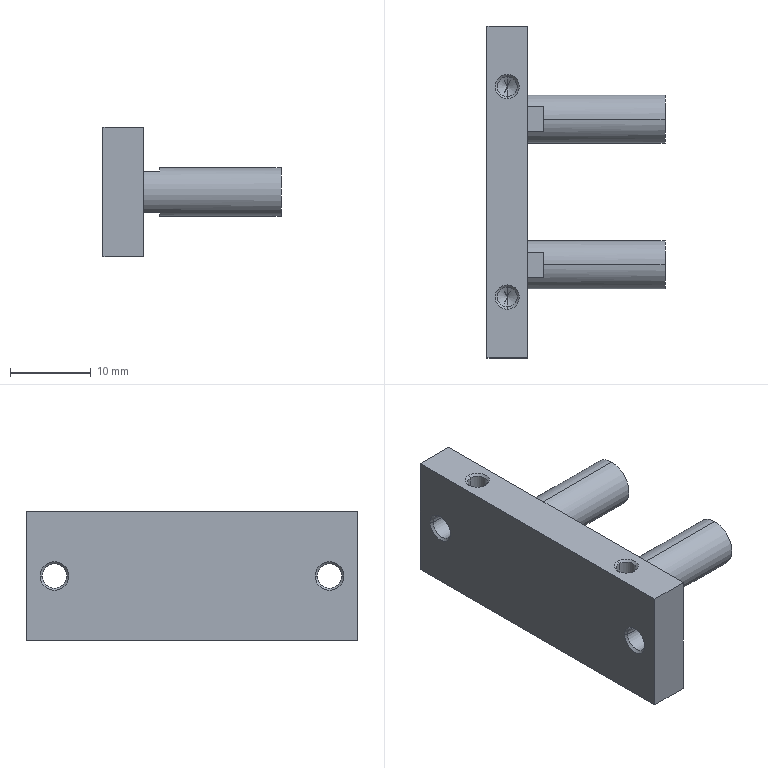Part | SolidWorks | features BaseBody 1 | 1 solid | 54 faces | box 22 x 41 x 16 mm | volume 4106 mm3 | cone 20 | plane 18 | cylinder 16 | commonest cylinder face diameters 2.459 x8 3 x4 6 x4
STEP:
#1=CARTESIAN_POINT('',(10.,9.,3.));
#2=VERTEX_POINT('',#1);
#3=CARTESIAN_POINT('',(10.,9.,-3.));
#4=VERTEX_POINT('',#3);
#5=CARTESIAN_POINT('',(10.,9.,0.));
#6=DIRECTION('',(1.,0.,0.));
#7=DIRECTION('',(0.,0.,-1.));
#8=AXIS2_PLACEMENT_3D('',#5,#6,#7);
#9=CIRCLE('',#8,3.);
#10=EDGE_CURVE('',#2,#4,#9,.T.);
#11=ORIENTED_EDGE('',*,*,#10,.F.);
#12=CARTESIAN_POINT('',(-5.,9.,3.));
#13=VERTEX_POINT('',#12);
#14=CARTESIAN_POINT('',(1.,9.,3.));
#15=DIRECTION('',(-1.,0.,0.));
#16=VECTOR('',#15,1000.);
#17=LINE('',#14,#16);
#18=EDGE_CURVE('',#2,#13,#17,.T.);
#19=ORIENTED_EDGE('',*,*,#18,.T.);
#20=CARTESIAN_POINT('',(-5.,7.42,2.55));
#21=VERTEX_POINT('',#20);
#22=CARTESIAN_POINT('',(-5.,9.,0.));
#23=DIRECTION('',(1.,0.,0.));
#24=DIRECTION('',(0.,0.,-1.));
#25=AXIS2_PLACEMENT_3D('',#22,#23,#24);
#26=CIRCLE('',#25,3.);
#27=EDGE_CURVE('',#13,#21,#26,.T.);
#28=ORIENTED_EDGE('',*,*,#27,.T.);
#29=CARTESIAN_POINT('',(-7.,7.42,2.55));
#30=VERTEX_POINT('',#29);
#31=CARTESIAN_POINT('',(-6.5,7.42,2.55));
#32=DIRECTION('',(-1.,0.,0.));
#33=VECTOR('',#32,1000.);
#34=LINE('',#31,#33);
#35=EDGE_CURVE('',#21,#30,#34,.T.);
#36=ORIENTED_EDGE('',*,*,#35,.T.);
#37=CARTESIAN_POINT('',(-7.,7.42,-2.55));
#38=VERTEX_POINT('',#37);
#39=CARTESIAN_POINT('',(-7.,9.,0.));
#40=DIRECTION('',(1.,0.,0.));
#41=DIRECTION('',(0.,0.,-1.));
#42=AXIS2_PLACEMENT_3D('',#39,#40,#41);
#43=CIRCLE('',#42,3.);
#44=EDGE_CURVE('',#30,#38,#43,.T.);
#45=ORIENTED_EDGE('',*,*,#44,.T.);
#46=CARTESIAN_POINT('',(-5.,7.42,-2.55));
#47=VERTEX_POINT('',#46);
#48=CARTESIAN_POINT('',(-6.5,7.42,-2.55));
#49=DIRECTION('',(1.,0.,0.));
#50=VECTOR('',#49,1000.);
#51=LINE('',#48,#50);
#52=EDGE_CURVE('',#38,#47,#51,.T.);
#53=ORIENTED_EDGE('',*,*,#52,.T.);
#54=CARTESIAN_POINT('',(-5.,9.,-3.));
#55=VERTEX_POINT('',#54);
#56=CARTESIAN_POINT('',(-5.,9.,0.));
#57=DIRECTION('',(1.,0.,0.));
#58=DIRECTION('',(0.,0.,-1.));
#59=AXIS2_PLACEMENT_3D('',#56,#57,#58);
#60=CIRCLE('',#59,3.);
#61=EDGE_CURVE('',#47,#55,#60,.T.);
#62=ORIENTED_EDGE('',*,*,#61,.T.);
#63=CARTESIAN_POINT('',(1.,9.,-3.));
#64=DIRECTION('',(-1.,0.,0.));
#65=VECTOR('',#64,1000.);
#66=LINE('',#63,#65);
#67=EDGE_CURVE('',#4,#55,#66,.T.);
#68=ORIENTED_EDGE('',*,*,#67,.F.);
#69=EDGE_LOOP('',(#11,#19,#28,#36,#45,#53,#62,#68));
#70=FACE_OUTER_BOUND('',#69,.T.);
#71=CARTESIAN_POINT('',(1.,9.,0.));
#72=DIRECTION('',(-1.,0.,0.));
#73=DIRECTION('',(0.,0.,-1.));
#74=AXIS2_PLACEMENT_3D('',#71,#72,#73);
#75=CYLINDRICAL_SURFACE('',#74,3.);
#76=ADVANCED_FACE('',(#70),#75,.T.);
#77=CARTESIAN_POINT('',(10.,-9.,3.));
#78=VERTEX_POINT('',#77);
#79=CARTESIAN_POINT('',(10.,-9.,-3.));
#80=VERTEX_POINT('',#79);
#81=CARTESIAN_POINT('',(10.,-9.,0.));
#82=DIRECTION('',(1.,0.,0.));
#83=DIRECTION('',(0.,0.,-1.));
#84=AXIS2_PLACEMENT_3D('',#81,#82,#83);
#85=CIRCLE('',#84,3.);
#86=EDGE_CURVE('',#78,#80,#85,.T.);
#87=ORIENTED_EDGE('',*,*,#86,.F.);
#88=CARTESIAN_POINT('',(-5.,-9.,3.));
#89=VERTEX_POINT('',#88);
#90=CARTESIAN_POINT('',(1.,-9.,3.));
#91=DIRECTION('',(-1.,0.,0.));
#92=VECTOR('',#91,1000.);
#93=LINE('',#90,#92);
#94=EDGE_CURVE('',#78,#89,#93,.T.);
#95=ORIENTED_EDGE('',*,*,#94,.T.);
#96=CARTESIAN_POINT('',(-5.,-10.58,2.55));
#97=VERTEX_POINT('',#96);
#98=CARTESIAN_POINT('',(-5.,-9.,0.));
#99=DIRECTION('',(1.,0.,0.));
#100=DIRECTION('',(0.,0.,-1.));
#101=AXIS2_PLACEMENT_3D('',#98,#99,#100);
#102=CIRCLE('',#101,3.);
#103=EDGE_CURVE('',#89,#97,#102,.T.);
#104=ORIENTED_EDGE('',*,*,#103,.T.);
#105=CARTESIAN_POINT('',(-7.,-10.58,2.55));
#106=VERTEX_POINT('',#105);
#107=CARTESIAN_POINT('',(-6.5,-10.58,2.55));
#108=DIRECTION('',(-1.,0.,0.));
#109=VECTOR('',#108,1000.);
#110=LINE('',#107,#109);
#111=EDGE_CURVE('',#97,#106,#110,.T.);
#112=ORIENTED_EDGE('',*,*,#111,.T.);
#113=CARTESIAN_POINT('',(-7.,-10.58,-2.55));
#114=VERTEX_POINT('',#113);
#115=CARTESIAN_POINT('',(-7.,-9.,0.));
#116=DIRECTION('',(-1.,0.,0.));
#117=DIRECTION('',(0.,0.,-1.));
#118=AXIS2_PLACEMENT_3D('',#115,#116,#117);
#119=CIRCLE('',#118,3.);
#120=EDGE_CURVE('',#114,#106,#119,.T.);
#121=ORIENTED_EDGE('',*,*,#120,.F.);
#122=CARTESIAN_POINT('',(-5.,-10.58,-2.55));
#123=VERTEX_POINT('',#122);
#124=CARTESIAN_POINT('',(-6.5,-10.58,-2.55));
#125=DIRECTION('',(1.,0.,0.));
#126=VECTOR('',#125,1000.);
#127=LINE('',#124,#126);
#128=EDGE_CURVE('',#114,#123,#127,.T.);
#129=ORIENTED_EDGE('',*,*,#128,.T.);
#130=CARTESIAN_POINT('',(-5.,-9.,-3.));
#131=VERTEX_POINT('',#130);
#132=CARTESIAN_POINT('',(-5.,-9.,0.));
#133=DIRECTION('',(1.,0.,0.));
#134=DIRECTION('',(0.,0.,-1.));
#135=AXIS2_PLACEMENT_3D('',#132,#133,#134);
#136=CIRCLE('',#135,3.);
#137=EDGE_CURVE('',#123,#131,#136,.T.);
#138=ORIENTED_EDGE('',*,*,#137,.T.);
#139=CARTESIAN_POINT('',(1.,-9.,-3.));
#140=DIRECTION('',(-1.,0.,0.));
#141=VECTOR('',#140,1000.);
#142=LINE('',#139,#141);
#143=EDGE_CURVE('',#80,#131,#142,.T.);
#144=ORIENTED_EDGE('',*,*,#143,.F.);
#145=EDGE_LOOP('',(#87,#95,#104,#112,#121,#129,#138,#144));
#146=FACE_OUTER_BOUND('',#145,.T.);
#147=CARTESIAN_POINT('',(1.,-9.,0.));
#148=DIRECTION('',(-1.,0.,0.));
#149=DIRECTION('',(0.,0.,-1.));
#150=AXIS2_PLACEMENT_3D('',#147,#148,#149);
#151=CYLINDRICAL_SURFACE('',#150,3.);
#152=ADVANCED_FACE('',(#146),#151,.T.);
#153=CARTESIAN_POINT('',(-9.5,13.,1.79));
#154=VERTEX_POINT('',#153);
#155=CARTESIAN_POINT('',(-9.5,14.229,2.5));
#156=VERTEX_POINT('',#155);
#157=CARTESIAN_POINT('',(-9.5,13.615,2.145));
#158=DIRECTION('',(0.,0.866,0.5));
#159=VECTOR('',#158,1000.);
#160=LINE('',#157,#159);
#161=EDGE_CURVE('',#154,#156,#160,.T.);
#162=ORIENTED_EDGE('',*,*,#161,.F.);
#163=CARTESIAN_POINT('',(-9.5,11.771,2.5));
#164=VERTEX_POINT('',#163);
#165=CARTESIAN_POINT('',(-9.5,12.385,2.145));
#166=DIRECTION('',(0.,-0.866,0.5));
#167=VECTOR('',#166,1000.);
#168=LINE('',#165,#167);
#169=EDGE_CURVE('',#154,#164,#168,.T.);
#170=ORIENTED_EDGE('',*,*,#169,.T.);
#171=CARTESIAN_POINT('',(-9.5,13.,2.5));
#172=DIRECTION('',(0.,0.,-1.));
#173=DIRECTION('',(0.,1.,0.));
#174=AXIS2_PLACEMENT_3D('',#171,#172,#173);
#175=CIRCLE('',#174,1.229);
#176=EDGE_CURVE('',#156,#164,#175,.T.);
#177=ORIENTED_EDGE('',*,*,#176,.F.);
#178=EDGE_LOOP('',(#162,#170,#177));
#179=FACE_OUTER_BOUND('',#178,.T.);
#180=CARTESIAN_POINT('',(-9.5,13.,2.145));
#181=DIRECTION('',(0.,0.,1.));
#182=DIRECTION('',(0.,1.,0.));
#183=AXIS2_PLACEMENT_3D('',#180,#181,#182);
#184=CONICAL_SURFACE('',#183,0.6147,1.047);
#185=ADVANCED_FACE('',(#179),#184,.F.);
#186=ORIENTED_EDGE('',*,*,#176,.T.);
#187=CARTESIAN_POINT('',(-9.5,11.771,3.729));
#188=VERTEX_POINT('',#187);
#189=CARTESIAN_POINT('',(-9.5,11.771,3.115));
#190=DIRECTION('',(0.,0.,1.));
#191=VECTOR('',#190,1000.);
#192=LINE('',#189,#191);
#193=EDGE_CURVE('',#164,#188,#192,.T.);
#194=ORIENTED_EDGE('',*,*,#193,.T.);
#195=CARTESIAN_POINT('',(-9.5,14.229,3.729));
#196=VERTEX_POINT('',#195);
#197=CARTESIAN_POINT('',(-9.5,13.,3.729));
#198=DIRECTION('',(0.,0.,-1.));
#199=DIRECTION('',(0.,1.,0.));
#200=AXIS2_PLACEMENT_3D('',#197,#198,#199);
#201=CIRCLE('',#200,1.229);
#202=EDGE_CURVE('',#196,#188,#201,.T.);
#203=ORIENTED_EDGE('',*,*,#202,.F.);
#204=CARTESIAN_POINT('',(-9.5,14.229,3.115));
#205=DIRECTION('',(0.,0.,1.));
#206=VECTOR('',#205,1000.);
#207=LINE('',#204,#206);
#208=EDGE_CURVE('',#156,#196,#207,.T.);
#209=ORIENTED_EDGE('',*,*,#208,.F.);
#210=EDGE_LOOP('',(#186,#194,#203,#209));
#211=FACE_OUTER_BOUND('',#210,.T.);
#212=CARTESIAN_POINT('',(-9.5,13.,3.115));
#213=DIRECTION('',(0.,0.,1.));
#214=DIRECTION('',(0.,1.,0.));
#215=AXIS2_PLACEMENT_3D('',#212,#213,#214);
#216=CYLINDRICAL_SURFACE('',#215,1.229);
#217=ADVANCED_FACE('',(#211),#216,.F.);
#218=ORIENTED_EDGE('',*,*,#202,.T.);
#219=CARTESIAN_POINT('',(-9.5,11.5,4.));
#220=VERTEX_POINT('',#219);
#221=CARTESIAN_POINT('',(-9.5,11.635,3.865));
#222=DIRECTION('',(0.,-0.7071,0.7071));
#223=VECTOR('',#222,1000.);
#224=LINE('',#221,#223);
#225=EDGE_CURVE('',#188,#220,#224,.T.);
#226=ORIENTED_EDGE('',*,*,#225,.T.);
#227=CARTESIAN_POINT('',(-9.5,14.5,4.));
#228=VERTEX_POINT('',#227);
#229=CARTESIAN_POINT('',(-9.5,13.,4.));
#230=DIRECTION('',(0.,0.,-1.));
#231=DIRECTION('',(0.,1.,0.));
#232=AXIS2_PLACEMENT_3D('',#229,#230,#231);
#233=CIRCLE('',#232,1.5);
#234=EDGE_CURVE('',#228,#220,#233,.T.);
#235=ORIENTED_EDGE('',*,*,#234,.F.);
#236=CARTESIAN_POINT('',(-9.5,14.365,3.865));
#237=DIRECTION('',(0.,0.7071,0.7071));
#238=VECTOR('',#237,1000.);
#239=LINE('',#236,#238);
#240=EDGE_CURVE('',#196,#228,#239,.T.);
#241=ORIENTED_EDGE('',*,*,#240,.F.);
#242=EDGE_LOOP('',(#218,#226,#235,#241));
#243=FACE_OUTER_BOUND('',#242,.T.);
#244=CARTESIAN_POINT('',(-9.5,13.,3.865));
#245=DIRECTION('',(0.,0.,1.));
#246=DIRECTION('',(0.,1.,0.));
#247=AXIS2_PLACEMENT_3D('',#244,#245,#246);
#248=CONICAL_SURFACE('',#247,1.365,0.7854);
#249=ADVANCED_FACE('',(#243),#248,.F.);
#250=CARTESIAN_POINT('',(-9.5,14.229,4.));
#251=VERTEX_POINT('',#250);
#252=CARTESIAN_POINT('',(-9.5,11.771,4.));
#253=VERTEX_POINT('',#252);
#254=CARTESIAN_POINT('',(-9.5,13.,4.));
#255=DIRECTION('',(0.,0.,-1.));
#256=DIRECTION('',(0.,1.,0.));
#257=AXIS2_PLACEMENT_3D('',#254,#255,#256);
#258=CIRCLE('',#257,1.229);
#259=EDGE_CURVE('',#251,#253,#258,.T.);
#260=ORIENTED_EDGE('',*,*,#259,.T.);
#261=CARTESIAN_POINT('',(-9.5,11.771,7.729));
#262=VERTEX_POINT('',#261);
#263=CARTESIAN_POINT('',(-9.5,11.771,5.865));
#264=DIRECTION('',(0.,0.,1.));
#265=VECTOR('',#264,1000.);
#266=LINE('',#263,#265);
#267=EDGE_CURVE('',#253,#262,#266,.T.);
#268=ORIENTED_EDGE('',*,*,#267,.T.);
#269=CARTESIAN_POINT('',(-9.5,14.229,7.729));
#270=VERTEX_POINT('',#269);
#271=CARTESIAN_POINT('',(-9.5,13.,7.729));
#272=DIRECTION('',(0.,0.,-1.));
#273=DIRECTION('',(0.,1.,0.));
#274=AXIS2_PLACEMENT_3D('',#271,#272,#273);
#275=CIRCLE('',#274,1.229);
#276=EDGE_CURVE('',#270,#262,#275,.T.);
#277=ORIENTED_EDGE('',*,*,#276,.F.);
#278=CARTESIAN_POINT('',(-9.5,14.229,5.865));
#279=DIRECTION('',(0.,0.,1.));
#280=VECTOR('',#279,1000.);
#281=LINE('',#278,#280);
#282=EDGE_CURVE('',#251,#270,#281,.T.);
#283=ORIENTED_EDGE('',*,*,#282,.F.);
#284=EDGE_LOOP('',(#260,#268,#277,#283));
#285=FACE_OUTER_BOUND('',#284,.T.);
#286=CARTESIAN_POINT('',(-9.5,13.,5.865));
#287=DIRECTION('',(0.,0.,1.));
#288=DIRECTION('',(0.,1.,0.));
#289=AXIS2_PLACEMENT_3D('',#286,#287,#288);
#290=CYLINDRICAL_SURFACE('',#289,1.229);
#291=ADVANCED_FACE('',(#285),#290,.F.);
#292=ORIENTED_EDGE('',*,*,#276,.T.);
#293=CARTESIAN_POINT('',(-9.5,11.5,8.));
#294=VERTEX_POINT('',#293);
#295=CARTESIAN_POINT('',(-9.5,11.635,7.865));
#296=DIRECTION('',(0.,-0.7071,0.7071));
#297=VECTOR('',#296,1000.);
#298=LINE('',#295,#297);
#299=EDGE_CURVE('',#262,#294,#298,.T.);
#300=ORIENTED_EDGE('',*,*,#299,.T.);
#301=CARTESIAN_POINT('',(-9.5,14.5,8.));
#302=VERTEX_POINT('',#301);
#303=CARTESIAN_POINT('',(-9.5,13.,8.));
#304=DIRECTION('',(0.,0.,-1.));
#305=DIRECTION('',(0.,1.,0.));
#306=AXIS2_PLACEMENT_3D('',#303,#304,#305);
#307=CIRCLE('',#306,1.5);
#308=EDGE_CURVE('',#302,#294,#307,.T.);
#309=ORIENTED_EDGE('',*,*,#308,.F.);
#310=CARTESIAN_POINT('',(-9.5,14.365,7.865));
#311=DIRECTION('',(0.,0.7071,0.7071));
#312=VECTOR('',#311,1000.);
#313=LINE('',#310,#312);
#314=EDGE_CURVE('',#270,#302,#313,.T.);
#315=ORIENTED_EDGE('',*,*,#314,.F.);
#316=EDGE_LOOP('',(#292,#300,#309,#315));
#317=FACE_OUTER_BOUND('',#316,.T.);
#318=CARTESIAN_POINT('',(-9.5,13.,7.865));
#319=DIRECTION('',(0.,0.,1.));
#320=DIRECTION('',(0.,1.,0.));
#321=AXIS2_PLACEMENT_3D('',#318,#319,#320);
#322=CONICAL_SURFACE('',#321,1.365,0.7854);
#323=ADVANCED_FACE('',(#317),#322,.F.);
#324=CARTESIAN_POINT('',(-9.5,-13.,1.79));
#325=VERTEX_POINT('',#324);
#326=CARTESIAN_POINT('',(-9.5,-11.771,2.5));
#327=VERTEX_POINT('',#326);
#328=CARTESIAN_POINT('',(-9.5,-12.385,2.145));
#329=DIRECTION('',(0.,0.866,0.5));
#330=VECTOR('',#329,1000.);
#331=LINE('',#328,#330);
#332=EDGE_CURVE('',#325,#327,#331,.T.);
#333=ORIENTED_EDGE('',*,*,#332,.F.);
#334=CARTESIAN_POINT('',(-9.5,-14.229,2.5));
#335=VERTEX_POINT('',#334);
#336=CARTESIAN_POINT('',(-9.5,-13.615,2.145));
#337=DIRECTION('',(0.,-0.866,0.5));
#338=VECTOR('',#337,1000.);
#339=LINE('',#336,#338);
#340=EDGE_CURVE('',#325,#335,#339,.T.);
#341=ORIENTED_EDGE('',*,*,#340,.T.);
#342=CARTESIAN_POINT('',(-9.5,-13.,2.5));
#343=DIRECTION('',(0.,0.,-1.));
#344=DIRECTION('',(0.,1.,0.));
#345=AXIS2_PLACEMENT_3D('',#342,#343,#344);
#346=CIRCLE('',#345,1.229);
#347=EDGE_CURVE('',#327,#335,#346,.T.);
#348=ORIENTED_EDGE('',*,*,#347,.F.);
#349=EDGE_LOOP('',(#333,#341,#348));
#350=FACE_OUTER_BOUND('',#349,.T.);
#351=CARTESIAN_POINT('',(-9.5,-13.,2.145));
#352=DIRECTION('',(0.,0.,1.));
#353=DIRECTION('',(0.,1.,0.));
#354=AXIS2_PLACEMENT_3D('',#351,#352,#353);
#355=CONICAL_SURFACE('',#354,0.6147,1.047);
#356=ADVANCED_FACE('',(#350),#355,.F.);
#357=ORIENTED_EDGE('',*,*,#347,.T.);
#358=CARTESIAN_POINT('',(-9.5,-14.229,3.729));
#359=VERTEX_POINT('',#358);
#360=CARTESIAN_POINT('',(-9.5,-14.229,3.115));
#361=DIRECTION('',(0.,0.,1.));
#362=VECTOR('',#361,1000.);
#363=LINE('',#360,#362);
#364=EDGE_CURVE('',#335,#359,#363,.T.);
#365=ORIENTED_EDGE('',*,*,#364,.T.);
#366=CARTESIAN_POINT('',(-9.5,-11.771,3.729));
#367=VERTEX_POINT('',#366);
#368=CARTESIAN_POINT('',(-9.5,-13.,3.729));
#369=DIRECTION('',(0.,0.,-1.));
#370=DIRECTION('',(0.,1.,0.));
#371=AXIS2_PLACEMENT_3D('',#368,#369,#370);
#372=CIRCLE('',#371,1.229);
#373=EDGE_CURVE('',#367,#359,#372,.T.);
#374=ORIENTED_EDGE('',*,*,#373,.F.);
#375=CARTESIAN_POINT('',(-9.5,-11.771,3.115));
#376=DIRECTION('',(0.,0.,1.));
#377=VECTOR('',#376,1000.);
#378=LINE('',#375,#377);
#379=EDGE_CURVE('',#327,#367,#378,.T.);
#380=ORIENTED_EDGE('',*,*,#379,.F.);
#381=EDGE_LOOP('',(#357,#365,#374,#380));
#382=FACE_OUTER_BOUND('',#381,.T.);
#383=CARTESIAN_POINT('',(-9.5,-13.,3.115));
#384=DIRECTION('',(0.,0.,1.));
#385=DIRECTION('',(0.,1.,0.));
#386=AXIS2_PLACEMENT_3D('',#383,#384,#385);
#387=CYLINDRICAL_SURFACE('',#386,1.229);
#388=ADVANCED_FACE('',(#382),#387,.F.);
#389=ORIENTED_EDGE('',*,*,#373,.T.);
#390=CARTESIAN_POINT('',(-9.5,-14.5,4.));
#391=VERTEX_POINT('',#390);
#392=CARTESIAN_POINT('',(-9.5,-14.365,3.865));
#393=DIRECTION('',(0.,-0.7071,0.7071));
#394=VECTOR('',#393,1000.);
#395=LINE('',#392,#394);
#396=EDGE_CURVE('',#359,#391,#395,.T.);
#397=ORIENTED_EDGE('',*,*,#396,.T.);
#398=CARTESIAN_POINT('',(-9.5,-11.5,4.));
#399=VERTEX_POINT('',#398);
#400=CARTESIAN_POINT('',(-9.5,-13.,4.));
#401=DIRECTION('',(0.,0.,-1.));
#402=DIRECTION('',(0.,1.,0.));
#403=AXIS2_PLACEMENT_3D('',#400,#401,#402);
#404=CIRCLE('',#403,1.5);
#405=EDGE_CURVE('',#399,#391,#404,.T.);
#406=ORIENTED_EDGE('',*,*,#405,.F.);
#407=CARTESIAN_POINT('',(-9.5,-11.635,3.865));
#408=DIRECTION('',(0.,0.7071,0.7071));
#409=VECTOR('',#408,1000.);
#410=LINE('',#407,#409);
#411=EDGE_CURVE('',#367,#399,#410,.T.);
#412=ORIENTED_EDGE('',*,*,#411,.F.);
#413=EDGE_LOOP('',(#389,#397,#406,#412));
#414=FACE_OUTER_BOUND('',#413,.T.);
#415=CARTESIAN_POINT('',(-9.5,-13.,3.865));
#416=DIRECTION('',(0.,0.,1.));
#417=DIRECTION('',(0.,1.,0.));
#418=AXIS2_PLACEMENT_3D('',#415,#416,#417);
#419=CONICAL_SURFACE('',#418,1.365,0.7854);
#420=ADVANCED_FACE('',(#414),#419,.F.);
#421=CARTESIAN_POINT('',(-9.5,-11.771,4.));
#422=VERTEX_POINT('',#421);
#423=CARTESIAN_POINT('',(-9.5,-14.229,4.));
#424=VERTEX_POINT('',#423);
#425=CARTESIAN_POINT('',(-9.5,-13.,4.));
#426=DIRECTION('',(0.,0.,-1.));
#427=DIRECTION('',(0.,1.,0.));
#428=AXIS2_PLACEMENT_3D('',#425,#426,#427);
#429=CIRCLE('',#428,1.229);
#430=EDGE_CURVE('',#422,#424,#429,.T.);
#431=ORIENTED_EDGE('',*,*,#430,.T.);
#432=CARTESIAN_POINT('',(-9.5,-14.229,7.729));
#433=VERTEX_POINT('',#432);
#434=CARTESIAN_POINT('',(-9.5,-14.229,5.865));
#435=DIRECTION('',(0.,0.,1.));
#436=VECTOR('',#435,1000.);
#437=LINE('',#434,#436);
#438=EDGE_CURVE('',#424,#433,#437,.T.);
#439=ORIENTED_EDGE('',*,*,#438,.T.);
#440=CARTESIAN_POINT('',(-9.5,-11.771,7.729));
#441=VERTEX_POINT('',#440);
#442=CARTESIAN_POINT('',(-9.5,-13.,7.729));
#443=DIRECTION('',(0.,0.,-1.));
#444=DIRECTION('',(0.,1.,0.));
#445=AXIS2_PLACEMENT_3D('',#442,#443,#444);
#446=CIRCLE('',#445,1.229);
#447=EDGE_CURVE('',#441,#433,#446,.T.);
#448=ORIENTED_EDGE('',*,*,#447,.F.);
#449=CARTESIAN_POINT('',(-9.5,-11.771,5.865));
#450=DIRECTION('',(0.,0.,1.));
#451=VECTOR('',#450,1000.);
#452=LINE('',#449,#451);
#453=EDGE_CURVE('',#422,#441,#452,.T.);
#454=ORIENTED_EDGE('',*,*,#453,.F.);
#455=EDGE_LOOP('',(#431,#439,#448,#454));
#456=FACE_OUTER_BOUND('',#455,.T.);
#457=CARTESIAN_POINT('',(-9.5,-13.,5.865));
#458=DIRECTION('',(0.,0.,1.));
#459=DIRECTION('',(0.,1.,0.));
#460=AXIS2_PLACEMENT_3D('',#457,#458,#459);
#461=CYLINDRICAL_SURFACE('',#460,1.229);
#462=ADVANCED_FACE('',(#456),#461,.F.);
#463=ORIENTED_EDGE('',*,*,#447,.T.);
#464=CARTESIAN_POINT('',(-9.5,-14.5,8.));
#465=VERTEX_POINT('',#464);
#466=CARTESIAN_POINT('',(-9.5,-14.365,7.865));
#467=DIRECTION('',(0.,-0.7071,0.7071));
#468=VECTOR('',#467,1000.);
#469=LINE('',#466,#468);
#470=EDGE_CURVE('',#433,#465,#469,.T.);
#471=ORIENTED_EDGE('',*,*,#470,.T.);
#472=CARTESIAN_POINT('',(-9.5,-11.5,8.));
#473=VERTEX_POINT('',#472);
#474=CARTESIAN_POINT('',(-9.5,-13.,8.));
#475=DIRECTION('',(0.,0.,-1.));
#476=DIRECTION('',(0.,1.,0.));
#477=AXIS2_PLACEMENT_3D('',#474,#475,#476);
#478=CIRCLE('',#477,1.5);
#479=EDGE_CURVE('',#473,#465,#478,.T.);
#480=ORIENTED_EDGE('',*,*,#479,.F.);
#481=CARTESIAN_POINT('',(-9.5,-11.635,7.865));
#482=DIRECTION('',(0.,0.7071,0.7071));
#483=VECTOR('',#482,1000.);
#484=LINE('',#481,#483);
#485=EDGE_CURVE('',#441,#473,#484,.T.);
#486=ORIENTED_EDGE('',*,*,#485,.F.);
#487=EDGE_LOOP('',(#463,#471,#480,#486));
#488=FACE_OUTER_BOUND('',#487,.T.);
#489=CARTESIAN_POINT('',(-9.5,-13.,7.865));
#490=DIRECTION('',(0.,0.,1.));
#491=DIRECTION('',(0.,1.,0.));
#492=AXIS2_PLACEMENT_3D('',#489,#490,#491);
#493=CONICAL_SURFACE('',#492,1.365,0.7854);
#494=ADVANCED_FACE('',(#488),#493,.F.);
#495=CARTESIAN_POINT('',(-7.271,-18.5,0.));
#496=VERTEX_POINT('',#495);
#497=CARTESIAN_POINT('',(-7.271,-15.5,0.));
#498=VERTEX_POINT('',#497);
#499=CARTESIAN_POINT('',(-7.271,-17.,0.));
#500=DIRECTION('',(1.,0.,0.));
#501=DIRECTION('',(0.,1.,0.));
#502=AXIS2_PLACEMENT_3D('',#499,#500,#501);
#503=CIRCLE('',#502,1.5);
#504=EDGE_CURVE('',#496,#498,#503,.T.);
#505=ORIENTED_EDGE('',*,*,#504,.F.);
#506=CARTESIAN_POINT('',(-7.,-18.771,0.));
#507=VERTEX_POINT('',#506);
#508=CARTESIAN_POINT('',(-7.135,-18.635,0.));
#509=DIRECTION('',(0.7071,-0.7071,0.));
#510=VECTOR('',#509,1000.);
#511=LINE('',#508,#510);
#512=EDGE_CURVE('',#496,#507,#511,.T.);
#513=ORIENTED_EDGE('',*,*,#512,.T.);
#514=CARTESIAN_POINT('',(-7.,-15.229,0.));
#515=VERTEX_POINT('',#514);
#516=CARTESIAN_POINT('',(-7.,-17.,0.));
#517=DIRECTION('',(-1.,0.,0.));
#518=DIRECTION('',(0.,1.,0.));
#519=AXIS2_PLACEMENT_3D('',#516,#517,#518);
#520=CIRCLE('',#519,1.771);
#521=EDGE_CURVE('',#515,#507,#520,.T.);
#522=ORIENTED_EDGE('',*,*,#521,.F.);
#523=CARTESIAN_POINT('',(-7.135,-15.365,0.));
#524=DIRECTION('',(0.7071,0.7071,0.));
#525=VECTOR('',#524,1000.);
#526=LINE('',#523,#525);
#527=EDGE_CURVE('',#498,#515,#526,.T.);
#528=ORIENTED_EDGE('',*,*,#527,.F.);
#529=EDGE_LOOP('',(#505,#513,#522,#528));
#530=FACE_OUTER_BOUND('',#529,.T.);
#531=CARTESIAN_POINT('',(-7.135,-17.,0.));
#532=DIRECTION('',(1.,0.,0.));
#533=DIRECTION('',(0.,1.,0.));
#534=AXIS2_PLACEMENT_3D('',#531,#532,#533);
#535=CONICAL_SURFACE('',#534,1.635,0.7854);
#536=ADVANCED_FACE('',(#530),#535,.F.);
#537=CARTESIAN_POINT('',(-7.271,-17.,0.));
#538=DIRECTION('',(1.,0.,0.));
#539=DIRECTION('',(0.,1.,0.));
#540=AXIS2_PLACEMENT_3D('',#537,#538,#539);
#541=CIRCLE('',#540,1.5);
#542=EDGE_CURVE('',#498,#496,#541,.T.);
#543=ORIENTED_EDGE('',*,*,#542,.T.);
#544=CARTESIAN_POINT('',(-11.729,-18.5,0.));
#545=VERTEX_POINT('',#544);
#546=CARTESIAN_POINT('',(-9.5,-18.5,0.));
#547=DIRECTION('',(-1.,0.,0.));
#548=VECTOR('',#547,1000.);
#549=LINE('',#546,#548);
#550=EDGE_CURVE('',#496,#545,#549,.T.);
#551=ORIENTED_EDGE('',*,*,#550,.T.);
#552=CARTESIAN_POINT('',(-11.729,-15.5,0.));
#553=VERTEX_POINT('',#552);
#554=CARTESIAN_POINT('',(-11.729,-17.,0.));
#555=DIRECTION('',(1.,0.,0.));
#556=DIRECTION('',(0.,1.,0.));
#557=AXIS2_PLACEMENT_3D('',#554,#555,#556);
#558=CIRCLE('',#557,1.5);
#559=EDGE_CURVE('',#553,#545,#558,.T.);
#560=ORIENTED_EDGE('',*,*,#559,.F.);
#561=CARTESIAN_POINT('',(-9.5,-15.5,0.));
#562=DIRECTION('',(-1.,0.,0.));
#563=VECTOR('',#562,1000.);
#564=LINE('',#561,#563);
#565=EDGE_CURVE('',#498,#553,#564,.T.);
#566=ORIENTED_EDGE('',*,*,#565,.F.);
#567=EDGE_LOOP('',(#543,#551,#560,#566));
#568=FACE_OUTER_BOUND('',#567,.T.);
#569=CARTESIAN_POINT('',(-9.5,-17.,0.));
#570=DIRECTION('',(-1.,0.,0.));
#571=DIRECTION('',(0.,1.,0.));
#572=AXIS2_PLACEMENT_3D('',#569,#570,#571);
#573=CYLINDRICAL_SURFACE('',#572,1.5);
#574=ADVANCED_FACE('',(#568),#573,.F.);
#575=ORIENTED_EDGE('',*,*,#559,.T.);
#576=CARTESIAN_POINT('',(-12.,-18.771,0.));
#577=VERTEX_POINT('',#576);
#578=CARTESIAN_POINT('',(-11.865,-18.635,0.));
#579=DIRECTION('',(-0.7071,-0.7071,0.));
#580=VECTOR('',#579,1000.);
#581=LINE('',#578,#580);
#582=EDGE_CURVE('',#545,#577,#581,.T.);
#583=ORIENTED_EDGE('',*,*,#582,.T.);
#584=CARTESIAN_POINT('',(-12.,-15.229,0.));
#585=VERTEX_POINT('',#584);
#586=CARTESIAN_POINT('',(-12.,-17.,0.));
#587=DIRECTION('',(1.,0.,0.));
#588=DIRECTION('',(0.,1.,0.));
#589=AXIS2_PLACEMENT_3D('',#586,#587,#588);
#590=CIRCLE('',#589,1.771);
#591=EDGE_CURVE('',#585,#577,#590,.T.);
#592=ORIENTED_EDGE('',*,*,#591,.F.);
#593=CARTESIAN_POINT('',(-11.865,-15.365,0.));
#594=DIRECTION('',(-0.7071,0.7071,0.));
#595=VECTOR('',#594,1000.);
#596=LINE('',#593,#595);
#597=EDGE_CURVE('',#553,#585,#596,.T.);
#598=ORIENTED_EDGE('',*,*,#597,.F.);
#599=EDGE_LOOP('',(#575,#583,#592,#598));
#600=FACE_OUTER_BOUND('',#599,.T.);
#601=CARTESIAN_POINT('',(-11.865,-17.,0.));
#602=DIRECTION('',(-1.,0.,0.));
#603=DIRECTION('',(0.,1.,0.));
#604=AXIS2_PLACEMENT_3D('',#601,#602,#603);
#605=CONICAL_SURFACE('',#604,1.635,0.7854);
#606=ADVANCED_FACE('',(#600),#605,.F.);
#607=CARTESIAN_POINT('',(-7.271,15.5,0.));
#608=VERTEX_POINT('',#607);
#609=CARTESIAN_POINT('',(-7.271,18.5,0.));
#610=VERTEX_POINT('',#609);
#611=CARTESIAN_POINT('',(-7.271,17.,0.));
#612=DIRECTION('',(1.,0.,0.));
#613=DIRECTION('',(0.,1.,0.));
#614=AXIS2_PLACEMENT_3D('',#611,#612,#613);
#615=CIRCLE('',#614,1.5);
#616=EDGE_CURVE('',#608,#610,#615,.T.);
#617=ORIENTED_EDGE('',*,*,#616,.F.);
#618=CARTESIAN_POINT('',(-7.,15.229,0.));
#619=VERTEX_POINT('',#618);
#620=CARTESIAN_POINT('',(-7.135,15.365,0.));
#621=DIRECTION('',(0.7071,-0.7071,0.));
#622=VECTOR('',#621,1000.);
#623=LINE('',#620,#622);
#624=EDGE_CURVE('',#608,#619,#623,.T.);
#625=ORIENTED_EDGE('',*,*,#624,.T.);
#626=CARTESIAN_POINT('',(-7.,18.771,0.));
#627=VERTEX_POINT('',#626);
#628=CARTESIAN_POINT('',(-7.,17.,0.));
#629=DIRECTION('',(-1.,0.,0.));
#630=DIRECTION('',(0.,1.,0.));
#631=AXIS2_PLACEMENT_3D('',#628,#629,#630);
#632=CIRCLE('',#631,1.771);
#633=EDGE_CURVE('',#627,#619,#632,.T.);
#634=ORIENTED_EDGE('',*,*,#633,.F.);
#635=CARTESIAN_POINT('',(-7.135,18.635,0.));
#636=DIRECTION('',(0.7071,0.7071,0.));
#637=VECTOR('',#636,1000.);
#638=LINE('',#635,#637);
#639=EDGE_CURVE('',#610,#627,#638,.T.);
#640=ORIENTED_EDGE('',*,*,#639,.F.);
#641=EDGE_LOOP('',(#617,#625,#634,#640));
#642=FACE_OUTER_BOUND('',#641,.T.);
#643=CARTESIAN_POINT('',(-7.135,17.,0.));
#644=DIRECTION('',(1.,0.,0.));
#645=DIRECTION('',(0.,1.,0.));
#646=AXIS2_PLACEMENT_3D('',#643,#644,#645);
#647=CONICAL_SURFACE('',#646,1.635,0.7854);
#648=ADVANCED_FACE('',(#642),#647,.F.);
#649=CARTESIAN_POINT('',(-7.271,17.,0.));
#650=DIRECTION('',(1.,0.,0.));
#651=DIRECTION('',(0.,1.,0.));
#652=AXIS2_PLACEMENT_3D('',#649,#650,#651);
#653=CIRCLE('',#652,1.5);
#654=EDGE_CURVE('',#610,#608,#653,.T.);
#655=ORIENTED_EDGE('',*,*,#654,.T.);
#656=CARTESIAN_POINT('',(-11.729,15.5,0.));
#657=VERTEX_POINT('',#656);
#658=CARTESIAN_POINT('',(-9.5,15.5,0.));
#659=DIRECTION('',(-1.,0.,0.));
#660=VECTOR('',#659,1000.);
#661=LINE('',#658,#660);
#662=EDGE_CURVE('',#608,#657,#661,.T.);
#663=ORIENTED_EDGE('',*,*,#662,.T.);
#664=CARTESIAN_POINT('',(-11.729,18.5,0.));
#665=VERTEX_POINT('',#664);
#666=CARTESIAN_POINT('',(-11.729,17.,0.));
#667=DIRECTION('',(1.,0.,0.));
#668=DIRECTION('',(0.,1.,0.));
#669=AXIS2_PLACEMENT_3D('',#666,#667,#668);
#670=CIRCLE('',#669,1.5);
#671=EDGE_CURVE('',#665,#657,#670,.T.);
#672=ORIENTED_EDGE('',*,*,#671,.F.);
#673=CARTESIAN_POINT('',(-9.5,18.5,0.));
#674=DIRECTION('',(-1.,0.,0.));
#675=VECTOR('',#674,1000.);
#676=LINE('',#673,#675);
#677=EDGE_CURVE('',#610,#665,#676,.T.);
#678=ORIENTED_EDGE('',*,*,#677,.F.);
#679=EDGE_LOOP('',(#655,#663,#672,#678));
#680=FACE_OUTER_BOUND('',#679,.T.);
#681=CARTESIAN_POINT('',(-9.5,17.,0.));
#682=DIRECTION('',(-1.,0.,0.));
#683=DIRECTION('',(0.,1.,0.));
#684=AXIS2_PLACEMENT_3D('',#681,#682,#683);
#685=CYLINDRICAL_SURFACE('',#684,1.5);
#686=ADVANCED_FACE('',(#680),#685,.F.);
#687=ORIENTED_EDGE('',*,*,#671,.T.);
#688=CARTESIAN_POINT('',(-12.,15.229,0.));
#689=VERTEX_POINT('',#688);
#690=CARTESIAN_POINT('',(-11.865,15.365,0.));
#691=DIRECTION('',(-0.7071,-0.7071,0.));
#692=VECTOR('',#691,1000.);
#693=LINE('',#690,#692);
#694=EDGE_CURVE('',#657,#689,#693,.T.);
#695=ORIENTED_EDGE('',*,*,#694,.T.);
#696=CARTESIAN_POINT('',(-12.,18.771,0.));
#697=VERTEX_POINT('',#696);
#698=CARTESIAN_POINT('',(-12.,17.,0.));
#699=DIRECTION('',(1.,0.,0.));
#700=DIRECTION('',(0.,1.,0.));
#701=AXIS2_PLACEMENT_3D('',#698,#699,#700);
#702=CIRCLE('',#701,1.771);
#703=EDGE_CURVE('',#697,#689,#702,.T.);
#704=ORIENTED_EDGE('',*,*,#703,.F.);
#705=CARTESIAN_POINT('',(-11.865,18.635,0.));
#706=DIRECTION('',(-0.7071,0.7071,0.));
#707=VECTOR('',#706,1000.);
#708=LINE('',#705,#707);
#709=EDGE_CURVE('',#665,#697,#708,.T.);
#710=ORIENTED_EDGE('',*,*,#709,.F.);
#711=EDGE_LOOP('',(#687,#695,#704,#710));
#712=FACE_OUTER_BOUND('',#711,.T.);
#713=CARTESIAN_POINT('',(-11.865,17.,0.));
#714=DIRECTION('',(-1.,0.,0.));
#715=DIRECTION('',(0.,1.,0.));
#716=AXIS2_PLACEMENT_3D('',#713,#714,#715);
#717=CONICAL_SURFACE('',#716,1.635,0.7854);
#718=ADVANCED_FACE('',(#712),#717,.F.);
#719=ORIENTED_EDGE('',*,*,#694,.F.);
#720=CARTESIAN_POINT('',(-11.729,17.,0.));
#721=DIRECTION('',(1.,0.,0.));
#722=DIRECTION('',(0.,1.,0.));
#723=AXIS2_PLACEMENT_3D('',#720,#721,#722);
#724=CIRCLE('',#723,1.5);
#725=EDGE_CURVE('',#657,#665,#724,.T.);
#726=ORIENTED_EDGE('',*,*,#725,.T.);
#727=ORIENTED_EDGE('',*,*,#709,.T.);
#728=CARTESIAN_POINT('',(-12.,17.,0.));
#729=DIRECTION('',(1.,0.,0.));
#730=DIRECTION('',(0.,1.,0.));
#731=AXIS2_PLACEMENT_3D('',#728,#729,#730);
#732=CIRCLE('',#731,1.771);
#733=EDGE_CURVE('',#689,#697,#732,.T.);
#734=ORIENTED_EDGE('',*,*,#733,.F.);
#735=EDGE_LOOP('',(#719,#726,#727,#734));
#736=FACE_OUTER_BOUND('',#735,.T.);
#737=CARTESIAN_POINT('',(-11.865,17.,0.));
#738=DIRECTION('',(-1.,0.,0.));
#739=DIRECTION('',(0.,1.,0.));
#740=AXIS2_PLACEMENT_3D('',#737,#738,#739);
#741=CONICAL_SURFACE('',#740,1.635,0.7854);
#742=ADVANCED_FACE('',(#736),#741,.F.);
#743=ORIENTED_EDGE('',*,*,#662,.F.);
#744=ORIENTED_EDGE('',*,*,#616,.T.);
#745=ORIENTED_EDGE('',*,*,#677,.T.);
#746=ORIENTED_EDGE('',*,*,#725,.F.);
#747=EDGE_LOOP('',(#743,#744,#745,#746));
#748=FACE_OUTER_BOUND('',#747,.T.);
#749=CARTESIAN_POINT('',(-9.5,17.,0.));
#750=DIRECTION('',(-1.,0.,0.));
#751=DIRECTION('',(0.,1.,0.));
#752=AXIS2_PLACEMENT_3D('',#749,#750,#751);
#753=CYLINDRICAL_SURFACE('',#752,1.5);
#754=ADVANCED_FACE('',(#748),#753,.F.);
#755=ORIENTED_EDGE('',*,*,#624,.F.);
#756=ORIENTED_EDGE('',*,*,#654,.F.);
#757=ORIENTED_EDGE('',*,*,#639,.T.);
#758=CARTESIAN_POINT('',(-7.,17.,0.));
#759=DIRECTION('',(-1.,0.,0.));
#760=DIRECTION('',(0.,1.,0.));
#761=AXIS2_PLACEMENT_3D('',#758,#759,#760);
#762=CIRCLE('',#761,1.771);
#763=EDGE_CURVE('',#619,#627,#762,.T.);
#764=ORIENTED_EDGE('',*,*,#763,.F.);
#765=EDGE_LOOP('',(#755,#756,#757,#764));
#766=FACE_OUTER_BOUND('',#765,.T.);
#767=CARTESIAN_POINT('',(-7.135,17.,0.));
#768=DIRECTION('',(1.,0.,0.));
#769=DIRECTION('',(0.,1.,0.));
#770=AXIS2_PLACEMENT_3D('',#767,#768,#769);
#771=CONICAL_SURFACE('',#770,1.635,0.7854);
#772=ADVANCED_FACE('',(#766),#771,.F.);
#773=ORIENTED_EDGE('',*,*,#582,.F.);
#774=CARTESIAN_POINT('',(-11.729,-17.,0.));
#775=DIRECTION('',(1.,0.,0.));
#776=DIRECTION('',(0.,1.,0.));
#777=AXIS2_PLACEMENT_3D('',#774,#775,#776);
#778=CIRCLE('',#777,1.5);
#779=EDGE_CURVE('',#545,#553,#778,.T.);
#780=ORIENTED_EDGE('',*,*,#779,.T.);
#781=ORIENTED_EDGE('',*,*,#597,.T.);
#782=CARTESIAN_POINT('',(-12.,-17.,0.));
#783=DIRECTION('',(1.,0.,0.));
#784=DIRECTION('',(0.,1.,0.));
#785=AXIS2_PLACEMENT_3D('',#782,#783,#784);
#786=CIRCLE('',#785,1.771);
#787=EDGE_CURVE('',#577,#585,#786,.T.);
#788=ORIENTED_EDGE('',*,*,#787,.F.);
#789=EDGE_LOOP('',(#773,#780,#781,#788));
#790=FACE_OUTER_BOUND('',#789,.T.);
#791=CARTESIAN_POINT('',(-11.865,-17.,0.));
#792=DIRECTION('',(-1.,0.,0.));
#793=DIRECTION('',(0.,1.,0.));
#794=AXIS2_PLACEMENT_3D('',#791,#792,#793);
#795=CONICAL_SURFACE('',#794,1.635,0.7854);
#796=ADVANCED_FACE('',(#790),#795,.F.);
#797=ORIENTED_EDGE('',*,*,#550,.F.);
#798=ORIENTED_EDGE('',*,*,#504,.T.);
#799=ORIENTED_EDGE('',*,*,#565,.T.);
#800=ORIENTED_EDGE('',*,*,#779,.F.);
#801=EDGE_LOOP('',(#797,#798,#799,#800));
#802=FACE_OUTER_BOUND('',#801,.T.);
#803=CARTESIAN_POINT('',(-9.5,-17.,0.));
#804=DIRECTION('',(-1.,0.,0.));
#805=DIRECTION('',(0.,1.,0.));
#806=AXIS2_PLACEMENT_3D('',#803,#804,#805);
#807=CYLINDRICAL_SURFACE('',#806,1.5);
#808=ADVANCED_FACE('',(#802),#807,.F.);
#809=ORIENTED_EDGE('',*,*,#512,.F.);
#810=ORIENTED_EDGE('',*,*,#542,.F.);
#811=ORIENTED_EDGE('',*,*,#527,.T.);
#812=CARTESIAN_POINT('',(-7.,-17.,0.));
#813=DIRECTION('',(-1.,0.,0.));
#814=DIRECTION('',(0.,1.,0.));
#815=AXIS2_PLACEMENT_3D('',#812,#813,#814);
#816=CIRCLE('',#815,1.771);
#817=EDGE_CURVE('',#507,#515,#816,.T.);
#818=ORIENTED_EDGE('',*,*,#817,.F.);
#819=EDGE_LOOP('',(#809,#810,#811,#818));
#820=FACE_OUTER_BOUND('',#819,.T.);
#821=CARTESIAN_POINT('',(-7.135,-17.,0.));
#822=DIRECTION('',(1.,0.,0.));
#823=DIRECTION('',(0.,1.,0.));
#824=AXIS2_PLACEMENT_3D('',#821,#822,#823);
#825=CONICAL_SURFACE('',#824,1.635,0.7854);
#826=ADVANCED_FACE('',(#820),#825,.F.);
#827=ORIENTED_EDGE('',*,*,#470,.F.);
#828=CARTESIAN_POINT('',(-9.5,-13.,7.729));
#829=DIRECTION('',(0.,0.,-1.));
#830=DIRECTION('',(0.,1.,0.));
#831=AXIS2_PLACEMENT_3D('',#828,#829,#830);
#832=CIRCLE('',#831,1.229);
#833=EDGE_CURVE('',#433,#441,#832,.T.);
#834=ORIENTED_EDGE('',*,*,#833,.T.);
#835=ORIENTED_EDGE('',*,*,#485,.T.);
#836=CARTESIAN_POINT('',(-9.5,-13.,8.));
#837=DIRECTION('',(0.,0.,-1.));
#838=DIRECTION('',(0.,1.,0.));
#839=AXIS2_PLACEMENT_3D('',#836,#837,#838);
#840=CIRCLE('',#839,1.5);
#841=EDGE_CURVE('',#465,#473,#840,.T.);
#842=ORIENTED_EDGE('',*,*,#841,.F.);
#843=EDGE_LOOP('',(#827,#834,#835,#842));
#844=FACE_OUTER_BOUND('',#843,.T.);
#845=CARTESIAN_POINT('',(-9.5,-13.,7.865));
#846=DIRECTION('',(0.,0.,1.));
#847=DIRECTION('',(0.,1.,0.));
#848=AXIS2_PLACEMENT_3D('',#845,#846,#847);
#849=CONICAL_SURFACE('',#848,1.365,0.7854);
#850=ADVANCED_FACE('',(#844),#849,.F.);
#851=ORIENTED_EDGE('',*,*,#438,.F.);
#852=CARTESIAN_POINT('',(-9.5,-13.,4.));
#853=DIRECTION('',(0.,0.,-1.));
#854=DIRECTION('',(0.,1.,0.));
#855=AXIS2_PLACEMENT_3D('',#852,#853,#854);
#856=CIRCLE('',#855,1.229);
#857=EDGE_CURVE('',#424,#422,#856,.T.);
#858=ORIENTED_EDGE('',*,*,#857,.T.);
#859=ORIENTED_EDGE('',*,*,#453,.T.);
#860=ORIENTED_EDGE('',*,*,#833,.F.);
#861=EDGE_LOOP('',(#851,#858,#859,#860));
#862=FACE_OUTER_BOUND('',#861,.T.);
#863=CARTESIAN_POINT('',(-9.5,-13.,5.865));
#864=DIRECTION('',(0.,0.,1.));
#865=DIRECTION('',(0.,1.,0.));
#866=AXIS2_PLACEMENT_3D('',#863,#864,#865);
#867=CYLINDRICAL_SURFACE('',#866,1.229);
#868=ADVANCED_FACE('',(#862),#867,.F.);
#869=ORIENTED_EDGE('',*,*,#405,.T.);
#870=CARTESIAN_POINT('',(-9.5,-13.,4.));
#871=DIRECTION('',(0.,0.,-1.));
#872=DIRECTION('',(0.,1.,0.));
#873=AXIS2_PLACEMENT_3D('',#870,#871,#872);
#874=CIRCLE('',#873,1.5);
#875=EDGE_CURVE('',#391,#399,#874,.T.);
#876=ORIENTED_EDGE('',*,*,#875,.T.);
#877=EDGE_LOOP('',(#869,#876));
#878=FACE_OUTER_BOUND('',#877,.T.);
#879=ORIENTED_EDGE('',*,*,#430,.F.);
#880=ORIENTED_EDGE('',*,*,#857,.F.);
#881=EDGE_LOOP('',(#879,#880));
#882=FACE_BOUND('',#881,.T.);
#883=CARTESIAN_POINT('',(-9.5,-11.635,4.));
#884=DIRECTION('',(0.,0.,1.));
#885=DIRECTION('',(0.,-1.,0.));
#886=AXIS2_PLACEMENT_3D('',#883,#884,#885);
#887=PLANE('',#886);
#888=ADVANCED_FACE('',(#878,#882),#887,.F.);
#889=ORIENTED_EDGE('',*,*,#396,.F.);
#890=CARTESIAN_POINT('',(-9.5,-13.,3.729));
#891=DIRECTION('',(0.,0.,-1.));
#892=DIRECTION('',(0.,1.,0.));
#893=AXIS2_PLACEMENT_3D('',#890,#891,#892);
#894=CIRCLE('',#893,1.229);
#895=EDGE_CURVE('',#359,#367,#894,.T.);
#896=ORIENTED_EDGE('',*,*,#895,.T.);
#897=ORIENTED_EDGE('',*,*,#411,.T.);
#898=ORIENTED_EDGE('',*,*,#875,.F.);
#899=EDGE_LOOP('',(#889,#896,#897,#898));
#900=FACE_OUTER_BOUND('',#899,.T.);
#901=CARTESIAN_POINT('',(-9.5,-13.,3.865));
#902=DIRECTION('',(0.,0.,1.));
#903=DIRECTION('',(0.,1.,0.));
#904=AXIS2_PLACEMENT_3D('',#901,#902,#903);
#905=CONICAL_SURFACE('',#904,1.365,0.7854);
#906=ADVANCED_FACE('',(#900),#905,.F.);
#907=ORIENTED_EDGE('',*,*,#364,.F.);
#908=CARTESIAN_POINT('',(-9.5,-13.,2.5));
#909=DIRECTION('',(0.,0.,-1.));
#910=DIRECTION('',(0.,1.,0.));
#911=AXIS2_PLACEMENT_3D('',#908,#909,#910);
#912=CIRCLE('',#911,1.229);
#913=EDGE_CURVE('',#335,#327,#912,.T.);
#914=ORIENTED_EDGE('',*,*,#913,.T.);
#915=ORIENTED_EDGE('',*,*,#379,.T.);
#916=ORIENTED_EDGE('',*,*,#895,.F.);
#917=EDGE_LOOP('',(#907,#914,#915,#916));
#918=FACE_OUTER_BOUND('',#917,.T.);
#919=CARTESIAN_POINT('',(-9.5,-13.,3.115));
#920=DIRECTION('',(0.,0.,1.));
#921=DIRECTION('',(0.,1.,0.));
#922=AXIS2_PLACEMENT_3D('',#919,#920,#921);
#923=CYLINDRICAL_SURFACE('',#922,1.229);
#924=ADVANCED_FACE('',(#918),#923,.F.);
#925=ORIENTED_EDGE('',*,*,#340,.F.);
#926=ORIENTED_EDGE('',*,*,#332,.T.);
#927=ORIENTED_EDGE('',*,*,#913,.F.);
#928=EDGE_LOOP('',(#925,#926,#927));
#929=FACE_OUTER_BOUND('',#928,.T.);
#930=CARTESIAN_POINT('',(-9.5,-13.,2.145));
#931=DIRECTION('',(0.,0.,1.));
#932=DIRECTION('',(0.,1.,0.));
#933=AXIS2_PLACEMENT_3D('',#930,#931,#932);
#934=CONICAL_SURFACE('',#933,0.6147,1.047);
#935=ADVANCED_FACE('',(#929),#934,.F.);
#936=ORIENTED_EDGE('',*,*,#299,.F.);
#937=CARTESIAN_POINT('',(-9.5,13.,7.729));
#938=DIRECTION('',(0.,0.,-1.));
#939=DIRECTION('',(0.,1.,0.));
#940=AXIS2_PLACEMENT_3D('',#937,#938,#939);
#941=CIRCLE('',#940,1.229);
#942=EDGE_CURVE('',#262,#270,#941,.T.);
#943=ORIENTED_EDGE('',*,*,#942,.T.);
#944=ORIENTED_EDGE('',*,*,#314,.T.);
#945=CARTESIAN_POINT('',(-9.5,13.,8.));
#946=DIRECTION('',(0.,0.,-1.));
#947=DIRECTION('',(0.,1.,0.));
#948=AXIS2_PLACEMENT_3D('',#945,#946,#947);
#949=CIRCLE('',#948,1.5);
#950=EDGE_CURVE('',#294,#302,#949,.T.);
#951=ORIENTED_EDGE('',*,*,#950,.F.);
#952=EDGE_LOOP('',(#936,#943,#944,#951));
#953=FACE_OUTER_BOUND('',#952,.T.);
#954=CARTESIAN_POINT('',(-9.5,13.,7.865));
#955=DIRECTION('',(0.,0.,1.));
#956=DIRECTION('',(0.,1.,0.));
#957=AXIS2_PLACEMENT_3D('',#954,#955,#956);
#958=CONICAL_SURFACE('',#957,1.365,0.7854);
#959=ADVANCED_FACE('',(#953),#958,.F.);
#960=ORIENTED_EDGE('',*,*,#267,.F.);
#961=CARTESIAN_POINT('',(-9.5,13.,4.));
#962=DIRECTION('',(0.,0.,-1.));
#963=DIRECTION('',(0.,1.,0.));
#964=AXIS2_PLACEMENT_3D('',#961,#962,#963);
#965=CIRCLE('',#964,1.229);
#966=EDGE_CURVE('',#253,#251,#965,.T.);
#967=ORIENTED_EDGE('',*,*,#966,.T.);
#968=ORIENTED_EDGE('',*,*,#282,.T.);
#969=ORIENTED_EDGE('',*,*,#942,.F.);
#970=EDGE_LOOP('',(#960,#967,#968,#969));
#971=FACE_OUTER_BOUND('',#970,.T.);
#972=CARTESIAN_POINT('',(-9.5,13.,5.865));
#973=DIRECTION('',(0.,0.,1.));
#974=DIRECTION('',(0.,1.,0.));
#975=AXIS2_PLACEMENT_3D('',#972,#973,#974);
#976=CYLINDRICAL_SURFACE('',#975,1.229);
#977=ADVANCED_FACE('',(#971),#976,.F.);
#978=ORIENTED_EDGE('',*,*,#234,.T.);
#979=CARTESIAN_POINT('',(-9.5,13.,4.));
#980=DIRECTION('',(0.,0.,-1.));
#981=DIRECTION('',(0.,1.,0.));
#982=AXIS2_PLACEMENT_3D('',#979,#980,#981);
#983=CIRCLE('',#982,1.5);
#984=EDGE_CURVE('',#220,#228,#983,.T.);
#985=ORIENTED_EDGE('',*,*,#984,.T.);
#986=EDGE_LOOP('',(#978,#985));
#987=FACE_OUTER_BOUND('',#986,.T.);
#988=ORIENTED_EDGE('',*,*,#259,.F.);
#989=ORIENTED_EDGE('',*,*,#966,.F.);
#990=EDGE_LOOP('',(#988,#989));
#991=FACE_BOUND('',#990,.T.);
#992=CARTESIAN_POINT('',(-9.5,14.365,4.));
#993=DIRECTION('',(0.,0.,1.));
#994=DIRECTION('',(0.,-1.,0.));
#995=AXIS2_PLACEMENT_3D('',#992,#993,#994);
#996=PLANE('',#995);
#997=ADVANCED_FACE('',(#987,#991),#996,.F.);
#998=ORIENTED_EDGE('',*,*,#225,.F.);
#999=CARTESIAN_POINT('',(-9.5,13.,3.729));
#1000=DIRECTION('',(0.,0.,-1.));
#1001=DIRECTION('',(0.,1.,0.));
#1002=AXIS2_PLACEMENT_3D('',#999,#1000,#1001);
#1003=CIRCLE('',#1002,1.229);
#1004=EDGE_CURVE('',#188,#196,#1003,.T.);
#1005=ORIENTED_EDGE('',*,*,#1004,.T.);
#1006=ORIENTED_EDGE('',*,*,#240,.T.);
#1007=ORIENTED_EDGE('',*,*,#984,.F.);
#1008=EDGE_LOOP('',(#998,#1005,#1006,#1007));
#1009=FACE_OUTER_BOUND('',#1008,.T.);
#1010=CARTESIAN_POINT('',(-9.5,13.,3.865));
#1011=DIRECTION('',(0.,0.,1.));
#1012=DIRECTION('',(0.,1.,0.));
#1013=AXIS2_PLACEMENT_3D('',#1010,#1011,#1012);
#1014=CONICAL_SURFACE('',#1013,1.365,0.7854);
#1015=ADVANCED_FACE('',(#1009),#1014,.F.);
#1016=ORIENTED_EDGE('',*,*,#193,.F.);
#1017=CARTESIAN_POINT('',(-9.5,13.,2.5));
#1018=DIRECTION('',(0.,0.,-1.));
#1019=DIRECTION('',(0.,1.,0.));
#1020=AXIS2_PLACEMENT_3D('',#1017,#1018,#1019);
#1021=CIRCLE('',#1020,1.229);
#1022=EDGE_CURVE('',#164,#156,#1021,.T.);
#1023=ORIENTED_EDGE('',*,*,#1022,.T.);
#1024=ORIENTED_EDGE('',*,*,#208,.T.);
#1025=ORIENTED_EDGE('',*,*,#1004,.F.);
#1026=EDGE_LOOP('',(#1016,#1023,#1024,#1025));
#1027=FACE_OUTER_BOUND('',#1026,.T.);
#1028=CARTESIAN_POINT('',(-9.5,13.,3.115));
#1029=DIRECTION('',(0.,0.,1.));
#1030=DIRECTION('',(0.,1.,0.));
#1031=AXIS2_PLACEMENT_3D('',#1028,#1029,#1030);
#1032=CYLINDRICAL_SURFACE('',#1031,1.229);
#1033=ADVANCED_FACE('',(#1027),#1032,.F.);
#1034=ORIENTED_EDGE('',*,*,#169,.F.);
#1035=ORIENTED_EDGE('',*,*,#161,.T.);
#1036=ORIENTED_EDGE('',*,*,#1022,.F.);
#1037=EDGE_LOOP('',(#1034,#1035,#1036));
#1038=FACE_OUTER_BOUND('',#1037,.T.);
#1039=CARTESIAN_POINT('',(-9.5,13.,2.145));
#1040=DIRECTION('',(0.,0.,1.));
#1041=DIRECTION('',(0.,1.,0.));
#1042=AXIS2_PLACEMENT_3D('',#1039,#1040,#1041);
#1043=CONICAL_SURFACE('',#1042,0.6147,1.047);
#1044=ADVANCED_FACE('',(#1038),#1043,.F.);
#1045=ORIENTED_EDGE('',*,*,#94,.F.);
#1046=CARTESIAN_POINT('',(10.,-9.,0.));
#1047=DIRECTION('',(1.,0.,0.));
#1048=DIRECTION('',(0.,0.,-1.));
#1049=AXIS2_PLACEMENT_3D('',#1046,#1047,#1048);
#1050=CIRCLE('',#1049,3.);
#1051=EDGE_CURVE('',#80,#78,#1050,.T.);
#1052=ORIENTED_EDGE('',*,*,#1051,.F.);
#1053=ORIENTED_EDGE('',*,*,#143,.T.);
#1054=CARTESIAN_POINT('',(-5.,-7.42,-2.55));
#1055=VERTEX_POINT('',#1054);
#1056=CARTESIAN_POINT('',(-5.,-9.,0.));
#1057=DIRECTION('',(1.,0.,0.));
#1058=DIRECTION('',(0.,0.,-1.));
#1059=AXIS2_PLACEMENT_3D('',#1056,#1057,#1058);
#1060=CIRCLE('',#1059,3.);
#1061=EDGE_CURVE('',#131,#1055,#1060,.T.);
#1062=ORIENTED_EDGE('',*,*,#1061,.T.);
#1063=CARTESIAN_POINT('',(-7.,-7.42,-2.55));
#1064=VERTEX_POINT('',#1063);
#1065=CARTESIAN_POINT('',(-6.5,-7.42,-2.55));
#1066=DIRECTION('',(-1.,0.,0.));
#1067=VECTOR('',#1066,1000.);
#1068=LINE('',#1065,#1067);
#1069=EDGE_CURVE('',#1055,#1064,#1068,.T.);
#1070=ORIENTED_EDGE('',*,*,#1069,.T.);
#1071=CARTESIAN_POINT('',(-7.,-7.42,2.55));
#1072=VERTEX_POINT('',#1071);
#1073=CARTESIAN_POINT('',(-7.,-9.,0.));
#1074=DIRECTION('',(-1.,0.,0.));
#1075=DIRECTION('',(0.,0.,-1.));
#1076=AXIS2_PLACEMENT_3D('',#1073,#1074,#1075);
#1077=CIRCLE('',#1076,3.);
#1078=EDGE_CURVE('',#1072,#1064,#1077,.T.);
#1079=ORIENTED_EDGE('',*,*,#1078,.F.);
#1080=CARTESIAN_POINT('',(-5.,-7.42,2.55));
#1081=VERTEX_POINT('',#1080);
#1082=CARTESIAN_POINT('',(-6.5,-7.42,2.55));
#1083=DIRECTION('',(1.,0.,0.));
#1084=VECTOR('',#1083,1000.);
#1085=LINE('',#1082,#1084);
#1086=EDGE_CURVE('',#1072,#1081,#1085,.T.);
#1087=ORIENTED_EDGE('',*,*,#1086,.T.);
#1088=CARTESIAN_POINT('',(-5.,-9.,0.));
#1089=DIRECTION('',(1.,0.,0.));
#1090=DIRECTION('',(0.,0.,-1.));
#1091=AXIS2_PLACEMENT_3D('',#1088,#1089,#1090);
#1092=CIRCLE('',#1091,3.);
#1093=EDGE_CURVE('',#1081,#89,#1092,.T.);
#1094=ORIENTED_EDGE('',*,*,#1093,.T.);
#1095=EDGE_LOOP('',(#1045,#1052,#1053,#1062,#1070,#1079,#1087,#1094));
#1096=FACE_OUTER_BOUND('',#1095,.T.);
#1097=CARTESIAN_POINT('',(1.,-9.,0.));
#1098=DIRECTION('',(-1.,0.,0.));
#1099=DIRECTION('',(0.,0.,-1.));
#1100=AXIS2_PLACEMENT_3D('',#1097,#1098,#1099);
#1101=CYLINDRICAL_SURFACE('',#1100,3.);
#1102=ADVANCED_FACE('',(#1096),#1101,.T.);
#1103=CARTESIAN_POINT('',(-7.,-4.5,2.55));
#1104=DIRECTION('',(0.,1.,0.));
#1105=VECTOR('',#1104,1000.);
#1106=LINE('',#1103,#1105);
#1107=EDGE_CURVE('',#106,#1072,#1106,.T.);
#1108=ORIENTED_EDGE('',*,*,#1107,.F.);
#1109=ORIENTED_EDGE('',*,*,#111,.F.);
#1110=CARTESIAN_POINT('',(-5.,-9.,2.55));
#1111=DIRECTION('',(0.,-1.,0.));
#1112=VECTOR('',#1111,1000.);
#1113=LINE('',#1110,#1112);
#1114=EDGE_CURVE('',#1081,#97,#1113,.T.);
#1115=ORIENTED_EDGE('',*,*,#1114,.F.);
#1116=ORIENTED_EDGE('',*,*,#1086,.F.);
#1117=EDGE_LOOP('',(#1108,#1109,#1115,#1116));
#1118=FACE_OUTER_BOUND('',#1117,.T.);
#1119=CARTESIAN_POINT('',(-7.,-9.,2.55));
#1120=DIRECTION('',(0.,0.,1.));
#1121=DIRECTION('',(1.,0.,0.));
#1122=AXIS2_PLACEMENT_3D('',#1119,#1120,#1121);
#1123=PLANE('',#1122);
#1124=ADVANCED_FACE('',(#1118),#1123,.T.);
#1125=CARTESIAN_POINT('',(-7.,-4.5,-2.55));
#1126=DIRECTION('',(0.,-1.,0.));
#1127=VECTOR('',#1126,1000.);
#1128=LINE('',#1125,#1127);
#1129=EDGE_CURVE('',#1064,#114,#1128,.T.);
#1130=ORIENTED_EDGE('',*,*,#1129,.F.);
#1131=ORIENTED_EDGE('',*,*,#1069,.F.);
#1132=CARTESIAN_POINT('',(-5.,-9.,-2.55));
#1133=DIRECTION('',(0.,1.,0.));
#1134=VECTOR('',#1133,1000.);
#1135=LINE('',#1132,#1134);
#1136=EDGE_CURVE('',#123,#1055,#1135,.T.);
#1137=ORIENTED_EDGE('',*,*,#1136,.F.);
#1138=ORIENTED_EDGE('',*,*,#128,.F.);
#1139=EDGE_LOOP('',(#1130,#1131,#1137,#1138));
#1140=FACE_OUTER_BOUND('',#1139,.T.);
#1141=CARTESIAN_POINT('',(-7.,-9.,-2.55));
#1142=DIRECTION('',(0.,0.,-1.));
#1143=DIRECTION('',(1.,0.,0.));
#1144=AXIS2_PLACEMENT_3D('',#1141,#1142,#1143);
#1145=PLANE('',#1144);
#1146=ADVANCED_FACE('',(#1140),#1145,.T.);
#1147=ORIENTED_EDGE('',*,*,#137,.F.);
#1148=ORIENTED_EDGE('',*,*,#1136,.T.);
#1149=ORIENTED_EDGE('',*,*,#1061,.F.);
#1150=EDGE_LOOP('',(#1147,#1148,#1149));
#1151=FACE_OUTER_BOUND('',#1150,.T.);
#1152=CARTESIAN_POINT('',(-5.,-9.,-4.05));
#1153=DIRECTION('',(-1.,0.,0.));
#1154=DIRECTION('',(0.,0.,-1.));
#1155=AXIS2_PLACEMENT_3D('',#1152,#1153,#1154);
#1156=PLANE('',#1155);
#1157=ADVANCED_FACE('',(#1151),#1156,.T.);
#1158=ORIENTED_EDGE('',*,*,#1093,.F.);
#1159=ORIENTED_EDGE('',*,*,#1114,.T.);
#1160=ORIENTED_EDGE('',*,*,#103,.F.);
#1161=EDGE_LOOP('',(#1158,#1159,#1160));
#1162=FACE_OUTER_BOUND('',#1161,.T.);
#1163=CARTESIAN_POINT('',(-5.,-9.,4.05));
#1164=DIRECTION('',(-1.,0.,0.));
#1165=DIRECTION('',(0.,0.,1.));
#1166=AXIS2_PLACEMENT_3D('',#1163,#1164,#1165);
#1167=PLANE('',#1166);
#1168=ADVANCED_FACE('',(#1162),#1167,.T.);
#1169=ORIENTED_EDGE('',*,*,#1051,.T.);
#1170=ORIENTED_EDGE('',*,*,#86,.T.);
#1171=EDGE_LOOP('',(#1169,#1170));
#1172=FACE_OUTER_BOUND('',#1171,.T.);
#1173=CARTESIAN_POINT('',(10.,-9.,0.));
#1174=DIRECTION('',(1.,0.,0.));
#1175=DIRECTION('',(0.,0.,-1.));
#1176=AXIS2_PLACEMENT_3D('',#1173,#1174,#1175);
#1177=PLANE('',#1176);
#1178=ADVANCED_FACE('',(#1172),#1177,.T.);
#1179=ORIENTED_EDGE('',*,*,#633,.T.);
#1180=ORIENTED_EDGE('',*,*,#763,.T.);
#1181=EDGE_LOOP('',(#1179,#1180));
#1182=FACE_BOUND('',#1181,.T.);
#1183=ORIENTED_EDGE('',*,*,#521,.T.);
#1184=ORIENTED_EDGE('',*,*,#817,.T.);
#1185=EDGE_LOOP('',(#1183,#1184));
#1186=FACE_BOUND('',#1185,.T.);
#1187=ORIENTED_EDGE('',*,*,#1107,.T.);
#1188=ORIENTED_EDGE('',*,*,#1078,.T.);
#1189=ORIENTED_EDGE('',*,*,#1129,.T.);
#1190=ORIENTED_EDGE('',*,*,#120,.T.);
#1191=EDGE_LOOP('',(#1187,#1188,#1189,#1190));
#1192=FACE_BOUND('',#1191,.T.);
#1193=CARTESIAN_POINT('',(-7.,-20.5,8.));
#1194=VERTEX_POINT('',#1193);
#1195=CARTESIAN_POINT('',(-7.,-20.5,-8.));
#1196=VERTEX_POINT('',#1195);
#1197=CARTESIAN_POINT('',(-7.,-20.5,0.));
#1198=DIRECTION('',(0.,0.,-1.));
#1199=VECTOR('',#1198,1000.);
#1200=LINE('',#1197,#1199);
#1201=EDGE_CURVE('',#1194,#1196,#1200,.T.);
#1202=ORIENTED_EDGE('',*,*,#1201,.T.);
#1203=CARTESIAN_POINT('',(-7.,20.5,-8.));
#1204=VERTEX_POINT('',#1203);
#1205=CARTESIAN_POINT('',(-7.,0.,-8.));
#1206=DIRECTION('',(0.,-1.,0.));
#1207=VECTOR('',#1206,1000.);
#1208=LINE('',#1205,#1207);
#1209=EDGE_CURVE('',#1204,#1196,#1208,.T.);
#1210=ORIENTED_EDGE('',*,*,#1209,.F.);
#1211=CARTESIAN_POINT('',(-7.,20.5,8.));
#1212=VERTEX_POINT('',#1211);
#1213=CARTESIAN_POINT('',(-7.,20.5,0.));
#1214=DIRECTION('',(0.,0.,-1.));
#1215=VECTOR('',#1214,1000.);
#1216=LINE('',#1213,#1215);
#1217=EDGE_CURVE('',#1212,#1204,#1216,.T.);
#1218=ORIENTED_EDGE('',*,*,#1217,.F.);
#1219=CARTESIAN_POINT('',(-7.,0.,8.));
#1220=DIRECTION('',(0.,1.,0.));
#1221=VECTOR('',#1220,1000.);
#1222=LINE('',#1219,#1221);
#1223=EDGE_CURVE('',#1194,#1212,#1222,.T.);
#1224=ORIENTED_EDGE('',*,*,#1223,.F.);
#1225=EDGE_LOOP('',(#1202,#1210,#1218,#1224));
#1226=FACE_OUTER_BOUND('',#1225,.T.);
#1227=CARTESIAN_POINT('',(-7.,10.58,2.55));
#1228=VERTEX_POINT('',#1227);
#1229=CARTESIAN_POINT('',(-7.,4.5,2.55));
#1230=DIRECTION('',(0.,-1.,0.));
#1231=VECTOR('',#1230,1000.);
#1232=LINE('',#1229,#1231);
#1233=EDGE_CURVE('',#1228,#30,#1232,.T.);
#1234=ORIENTED_EDGE('',*,*,#1233,.F.);
#1235=CARTESIAN_POINT('',(-7.,10.58,-2.55));
#1236=VERTEX_POINT('',#1235);
#1237=CARTESIAN_POINT('',(-7.,9.,0.));
#1238=DIRECTION('',(1.,0.,0.));
#1239=DIRECTION('',(0.,0.,-1.));
#1240=AXIS2_PLACEMENT_3D('',#1237,#1238,#1239);
#1241=CIRCLE('',#1240,3.);
#1242=EDGE_CURVE('',#1236,#1228,#1241,.T.);
#1243=ORIENTED_EDGE('',*,*,#1242,.F.);
#1244=CARTESIAN_POINT('',(-7.,4.5,-2.55));
#1245=DIRECTION('',(0.,1.,0.));
#1246=VECTOR('',#1245,1000.);
#1247=LINE('',#1244,#1246);
#1248=EDGE_CURVE('',#38,#1236,#1247,.T.);
#1249=ORIENTED_EDGE('',*,*,#1248,.F.);
#1250=ORIENTED_EDGE('',*,*,#44,.F.);
#1251=EDGE_LOOP('',(#1234,#1243,#1249,#1250));
#1252=FACE_BOUND('',#1251,.T.);
#1253=CARTESIAN_POINT('',(-7.,0.,0.));
#1254=DIRECTION('',(-1.,0.,0.));
#1255=DIRECTION('',(0.,0.,1.));
#1256=AXIS2_PLACEMENT_3D('',#1253,#1254,#1255);
#1257=PLANE('',#1256);
#1258=ADVANCED_FACE('',(#1182,#1186,#1192,#1226,#1252),#1257,.F.);
#1259=ORIENTED_EDGE('',*,*,#479,.T.);
#1260=ORIENTED_EDGE('',*,*,#841,.T.);
#1261=EDGE_LOOP('',(#1259,#1260));
#1262=FACE_BOUND('',#1261,.T.);
#1263=ORIENTED_EDGE('',*,*,#308,.T.);
#1264=ORIENTED_EDGE('',*,*,#950,.T.);
#1265=EDGE_LOOP('',(#1263,#1264));
#1266=FACE_BOUND('',#1265,.T.);
#1267=ORIENTED_EDGE('',*,*,#1223,.T.);
#1268=CARTESIAN_POINT('',(-12.,20.5,8.));
#1269=VERTEX_POINT('',#1268);
#1270=CARTESIAN_POINT('',(-9.5,20.5,8.));
#1271=DIRECTION('',(-1.,0.,0.));
#1272=VECTOR('',#1271,1000.);
#1273=LINE('',#1270,#1272);
#1274=EDGE_CURVE('',#1212,#1269,#1273,.T.);
#1275=ORIENTED_EDGE('',*,*,#1274,.T.);
#1276=CARTESIAN_POINT('',(-12.,-20.5,8.));
#1277=VERTEX_POINT('',#1276);
#1278=CARTESIAN_POINT('',(-12.,0.,8.));
#1279=DIRECTION('',(0.,-1.,0.));
#1280=VECTOR('',#1279,1000.);
#1281=LINE('',#1278,#1280);
#1282=EDGE_CURVE('',#1269,#1277,#1281,.T.);
#1283=ORIENTED_EDGE('',*,*,#1282,.T.);
#1284=CARTESIAN_POINT('',(-9.5,-20.5,8.));
#1285=DIRECTION('',(1.,0.,0.));
#1286=VECTOR('',#1285,1000.);
#1287=LINE('',#1284,#1286);
#1288=EDGE_CURVE('',#1277,#1194,#1287,.T.);
#1289=ORIENTED_EDGE('',*,*,#1288,.T.);
#1290=EDGE_LOOP('',(#1267,#1275,#1283,#1289));
#1291=FACE_OUTER_BOUND('',#1290,.T.);
#1292=CARTESIAN_POINT('',(-9.5,0.,8.));
#1293=DIRECTION('',(0.,0.,1.));
#1294=DIRECTION('',(1.,0.,0.));
#1295=AXIS2_PLACEMENT_3D('',#1292,#1293,#1294);
#1296=PLANE('',#1295);
#1297=ADVANCED_FACE('',(#1262,#1266,#1291),#1296,.T.);
#1298=ORIENTED_EDGE('',*,*,#1209,.T.);
#1299=CARTESIAN_POINT('',(-12.,-20.5,-8.));
#1300=VERTEX_POINT('',#1299);
#1301=CARTESIAN_POINT('',(-9.5,-20.5,-8.));
#1302=DIRECTION('',(-1.,0.,0.));
#1303=VECTOR('',#1302,1000.);
#1304=LINE('',#1301,#1303);
#1305=EDGE_CURVE('',#1196,#1300,#1304,.T.);
#1306=ORIENTED_EDGE('',*,*,#1305,.T.);
#1307=CARTESIAN_POINT('',(-12.,20.5,-8.));
#1308=VERTEX_POINT('',#1307);
#1309=CARTESIAN_POINT('',(-12.,0.,-8.));
#1310=DIRECTION('',(0.,1.,0.));
#1311=VECTOR('',#1310,1000.);
#1312=LINE('',#1309,#1311);
#1313=EDGE_CURVE('',#1300,#1308,#1312,.T.);
#1314=ORIENTED_EDGE('',*,*,#1313,.T.);
#1315=CARTESIAN_POINT('',(-9.5,20.5,-8.));
#1316=DIRECTION('',(1.,0.,0.));
#1317=VECTOR('',#1316,1000.);
#1318=LINE('',#1315,#1317);
#1319=EDGE_CURVE('',#1308,#1204,#1318,.T.);
#1320=ORIENTED_EDGE('',*,*,#1319,.T.);
#1321=EDGE_LOOP('',(#1298,#1306,#1314,#1320));
#1322=FACE_OUTER_BOUND('',#1321,.T.);
#1323=CARTESIAN_POINT('',(-9.5,0.,-8.));
#1324=DIRECTION('',(0.,0.,1.));
#1325=DIRECTION('',(1.,0.,0.));
#1326=AXIS2_PLACEMENT_3D('',#1323,#1324,#1325);
#1327=PLANE('',#1326);
#1328=ADVANCED_FACE('',(#1322),#1327,.F.);
#1329=CARTESIAN_POINT('',(-12.,-20.5,0.));
#1330=DIRECTION('',(0.,0.,-1.));
#1331=VECTOR('',#1330,1000.);
#1332=LINE('',#1329,#1331);
#1333=EDGE_CURVE('',#1277,#1300,#1332,.T.);
#1334=ORIENTED_EDGE('',*,*,#1333,.T.);
#1335=ORIENTED_EDGE('',*,*,#1305,.F.);
#1336=ORIENTED_EDGE('',*,*,#1201,.F.);
#1337=ORIENTED_EDGE('',*,*,#1288,.F.);
#1338=EDGE_LOOP('',(#1334,#1335,#1336,#1337));
#1339=FACE_OUTER_BOUND('',#1338,.T.);
#1340=CARTESIAN_POINT('',(-9.5,-20.5,0.));
#1341=DIRECTION('',(0.,1.,0.));
#1342=DIRECTION('',(0.,0.,1.));
#1343=AXIS2_PLACEMENT_3D('',#1340,#1341,#1342);
#1344=PLANE('',#1343);
#1345=ADVANCED_FACE('',(#1339),#1344,.F.);
#1346=ORIENTED_EDGE('',*,*,#703,.T.);
#1347=ORIENTED_EDGE('',*,*,#733,.T.);
#1348=EDGE_LOOP('',(#1346,#1347));
#1349=FACE_BOUND('',#1348,.T.);
#1350=ORIENTED_EDGE('',*,*,#591,.T.);
#1351=ORIENTED_EDGE('',*,*,#787,.T.);
#1352=EDGE_LOOP('',(#1350,#1351));
#1353=FACE_BOUND('',#1352,.T.);
#1354=CARTESIAN_POINT('',(-12.,20.5,0.));
#1355=DIRECTION('',(0.,0.,-1.));
#1356=VECTOR('',#1355,1000.);
#1357=LINE('',#1354,#1356);
#1358=EDGE_CURVE('',#1269,#1308,#1357,.T.);
#1359=ORIENTED_EDGE('',*,*,#1358,.T.);
#1360=ORIENTED_EDGE('',*,*,#1313,.F.);
#1361=ORIENTED_EDGE('',*,*,#1333,.F.);
#1362=ORIENTED_EDGE('',*,*,#1282,.F.);
#1363=EDGE_LOOP('',(#1359,#1360,#1361,#1362));
#1364=FACE_OUTER_BOUND('',#1363,.T.);
#1365=CARTESIAN_POINT('',(-12.,0.,0.));
#1366=DIRECTION('',(1.,0.,0.));
#1367=DIRECTION('',(0.,0.,-1.));
#1368=AXIS2_PLACEMENT_3D('',#1365,#1366,#1367);
#1369=PLANE('',#1368);
#1370=ADVANCED_FACE('',(#1349,#1353,#1364),#1369,.F.);
#1371=ORIENTED_EDGE('',*,*,#1217,.T.);
#1372=ORIENTED_EDGE('',*,*,#1319,.F.);
#1373=ORIENTED_EDGE('',*,*,#1358,.F.);
#1374=ORIENTED_EDGE('',*,*,#1274,.F.);
#1375=EDGE_LOOP('',(#1371,#1372,#1373,#1374));
#1376=FACE_OUTER_BOUND('',#1375,.T.);
#1377=CARTESIAN_POINT('',(-9.5,20.5,0.));
#1378=DIRECTION('',(0.,-1.,0.));
#1379=DIRECTION('',(0.,0.,-1.));
#1380=AXIS2_PLACEMENT_3D('',#1377,#1378,#1379);
#1381=PLANE('',#1380);
#1382=ADVANCED_FACE('',(#1376),#1381,.F.);
#1383=ORIENTED_EDGE('',*,*,#1248,.T.);
#1384=CARTESIAN_POINT('',(-5.,10.58,-2.55));
#1385=VERTEX_POINT('',#1384);
#1386=CARTESIAN_POINT('',(-6.5,10.58,-2.55));
#1387=DIRECTION('',(-1.,0.,0.));
#1388=VECTOR('',#1387,1000.);
#1389=LINE('',#1386,#1388);
#1390=EDGE_CURVE('',#1385,#1236,#1389,.T.);
#1391=ORIENTED_EDGE('',*,*,#1390,.F.);
#1392=CARTESIAN_POINT('',(-5.,9.,-2.55));
#1393=DIRECTION('',(0.,1.,0.));
#1394=VECTOR('',#1393,1000.);
#1395=LINE('',#1392,#1394);
#1396=EDGE_CURVE('',#47,#1385,#1395,.T.);
#1397=ORIENTED_EDGE('',*,*,#1396,.F.);
#1398=ORIENTED_EDGE('',*,*,#52,.F.);
#1399=EDGE_LOOP('',(#1383,#1391,#1397,#1398));
#1400=FACE_OUTER_BOUND('',#1399,.T.);
#1401=CARTESIAN_POINT('',(-7.,9.,-2.55));
#1402=DIRECTION('',(0.,0.,-1.));
#1403=DIRECTION('',(1.,0.,0.));
#1404=AXIS2_PLACEMENT_3D('',#1401,#1402,#1403);
#1405=PLANE('',#1404);
#1406=ADVANCED_FACE('',(#1400),#1405,.T.);
#1407=ORIENTED_EDGE('',*,*,#61,.F.);
#1408=ORIENTED_EDGE('',*,*,#1396,.T.);
#1409=CARTESIAN_POINT('',(-5.,9.,0.));
#1410=DIRECTION('',(1.,0.,0.));
#1411=DIRECTION('',(0.,0.,-1.));
#1412=AXIS2_PLACEMENT_3D('',#1409,#1410,#1411);
#1413=CIRCLE('',#1412,3.);
#1414=EDGE_CURVE('',#55,#1385,#1413,.T.);
#1415=ORIENTED_EDGE('',*,*,#1414,.F.);
#1416=EDGE_LOOP('',(#1407,#1408,#1415));
#1417=FACE_OUTER_BOUND('',#1416,.T.);
#1418=CARTESIAN_POINT('',(-5.,9.,-4.05));
#1419=DIRECTION('',(-1.,0.,0.));
#1420=DIRECTION('',(0.,0.,-1.));
#1421=AXIS2_PLACEMENT_3D('',#1418,#1419,#1420);
#1422=PLANE('',#1421);
#1423=ADVANCED_FACE('',(#1417),#1422,.T.);
#1424=CARTESIAN_POINT('',(-5.,10.58,2.55));
#1425=VERTEX_POINT('',#1424);
#1426=CARTESIAN_POINT('',(-5.,9.,0.));
#1427=DIRECTION('',(1.,0.,0.));
#1428=DIRECTION('',(0.,0.,-1.));
#1429=AXIS2_PLACEMENT_3D('',#1426,#1427,#1428);
#1430=CIRCLE('',#1429,3.);
#1431=EDGE_CURVE('',#1425,#13,#1430,.T.);
#1432=ORIENTED_EDGE('',*,*,#1431,.F.);
#1433=CARTESIAN_POINT('',(-5.,9.,2.55));
#1434=DIRECTION('',(0.,-1.,0.));
#1435=VECTOR('',#1434,1000.);
#1436=LINE('',#1433,#1435);
#1437=EDGE_CURVE('',#1425,#21,#1436,.T.);
#1438=ORIENTED_EDGE('',*,*,#1437,.T.);
#1439=ORIENTED_EDGE('',*,*,#27,.F.);
#1440=EDGE_LOOP('',(#1432,#1438,#1439));
#1441=FACE_OUTER_BOUND('',#1440,.T.);
#1442=CARTESIAN_POINT('',(-5.,9.,4.05));
#1443=DIRECTION('',(-1.,0.,0.));
#1444=DIRECTION('',(0.,0.,1.));
#1445=AXIS2_PLACEMENT_3D('',#1442,#1443,#1444);
#1446=PLANE('',#1445);
#1447=ADVANCED_FACE('',(#1441),#1446,.T.);
#1448=ORIENTED_EDGE('',*,*,#1233,.T.);
#1449=ORIENTED_EDGE('',*,*,#35,.F.);
#1450=ORIENTED_EDGE('',*,*,#1437,.F.);
#1451=CARTESIAN_POINT('',(-6.5,10.58,2.55));
#1452=DIRECTION('',(1.,0.,0.));
#1453=VECTOR('',#1452,1000.);
#1454=LINE('',#1451,#1453);
#1455=EDGE_CURVE('',#1228,#1425,#1454,.T.);
#1456=ORIENTED_EDGE('',*,*,#1455,.F.);
#1457=EDGE_LOOP('',(#1448,#1449,#1450,#1456));
#1458=FACE_OUTER_BOUND('',#1457,.T.);
#1459=CARTESIAN_POINT('',(-7.,9.,2.55));
#1460=DIRECTION('',(0.,0.,1.));
#1461=DIRECTION('',(1.,0.,0.));
#1462=AXIS2_PLACEMENT_3D('',#1459,#1460,#1461);
#1463=PLANE('',#1462);
#1464=ADVANCED_FACE('',(#1458),#1463,.T.);
#1465=ORIENTED_EDGE('',*,*,#18,.F.);
#1466=CARTESIAN_POINT('',(10.,9.,0.));
#1467=DIRECTION('',(1.,0.,0.));
#1468=DIRECTION('',(0.,0.,-1.));
#1469=AXIS2_PLACEMENT_3D('',#1466,#1467,#1468);
#1470=CIRCLE('',#1469,3.);
#1471=EDGE_CURVE('',#4,#2,#1470,.T.);
#1472=ORIENTED_EDGE('',*,*,#1471,.F.);
#1473=ORIENTED_EDGE('',*,*,#67,.T.);
#1474=ORIENTED_EDGE('',*,*,#1414,.T.);
#1475=ORIENTED_EDGE('',*,*,#1390,.T.);
#1476=ORIENTED_EDGE('',*,*,#1242,.T.);
#1477=ORIENTED_EDGE('',*,*,#1455,.T.);
#1478=ORIENTED_EDGE('',*,*,#1431,.T.);
#1479=EDGE_LOOP('',(#1465,#1472,#1473,#1474,#1475,#1476,#1477,#1478));
#1480=FACE_OUTER_BOUND('',#1479,.T.);
#1481=CARTESIAN_POINT('',(1.,9.,0.));
#1482=DIRECTION('',(-1.,0.,0.));
#1483=DIRECTION('',(0.,0.,-1.));
#1484=AXIS2_PLACEMENT_3D('',#1481,#1482,#1483);
#1485=CYLINDRICAL_SURFACE('',#1484,3.);
#1486=ADVANCED_FACE('',(#1480),#1485,.T.);
#1487=ORIENTED_EDGE('',*,*,#1471,.T.);
#1488=ORIENTED_EDGE('',*,*,#10,.T.);
#1489=EDGE_LOOP('',(#1487,#1488));
#1490=FACE_OUTER_BOUND('',#1489,.T.);
#1491=CARTESIAN_POINT('',(10.,9.,0.));
#1492=DIRECTION('',(1.,0.,0.));
#1493=DIRECTION('',(0.,0.,-1.));
#1494=AXIS2_PLACEMENT_3D('',#1491,#1492,#1493);
#1495=PLANE('',#1494);
#1496=ADVANCED_FACE('',(#1490),#1495,.T.);
#1497=CLOSED_SHELL('',(#76,#152,#185,#217,#249,#291,#323,#356,#388,#420,#462,#494,#536,#574,#606,#648,#686,#718,#742,#754,#772,#796,#808,#826,#850,#868,#888,#906,#924,#935,#959,#977,#997,#1015,#1033,#1044,#1102,#1124,#1146,#1157,#1168,#1178,#1258,#1297,#1328,#1345,#1370,#1382,#1406,#1423,#1447,#1464,#1486,#1496));
#1498=MANIFOLD_SOLID_BREP('',#1497);
#1499=CARTESIAN_POINT('',(0.,0.,0.));
#1500=DIRECTION('',(0.,0.,1.));
#1501=DIRECTION('',(1.,0.,0.));
#1502=AXIS2_PLACEMENT_3D('',#1499,#1500,#1501);
#1503=(LENGTH_UNIT()NAMED_UNIT(*)SI_UNIT(.MILLI.,.METRE.));
#1504=UNCERTAINTY_MEASURE_WITH_UNIT(LENGTH_MEASURE(0.00001),#1503,'','');
#1505=(NAMED_UNIT(*)PLANE_ANGLE_UNIT()SI_UNIT($,.RADIAN.));
#1506=(NAMED_UNIT(*)SI_UNIT($,.STERADIAN.)SOLID_ANGLE_UNIT());
#1507=(GEOMETRIC_REPRESENTATION_CONTEXT(3)GLOBAL_UNCERTAINTY_ASSIGNED_CONTEXT((#1504))GLOBAL_UNIT_ASSIGNED_CONTEXT((#1503,#1505,#1506))REPRESENTATION_CONTEXT('',''));
#1508=ADVANCED_BREP_SHAPE_REPRESENTATION('',(#1498,#1502),#1507);